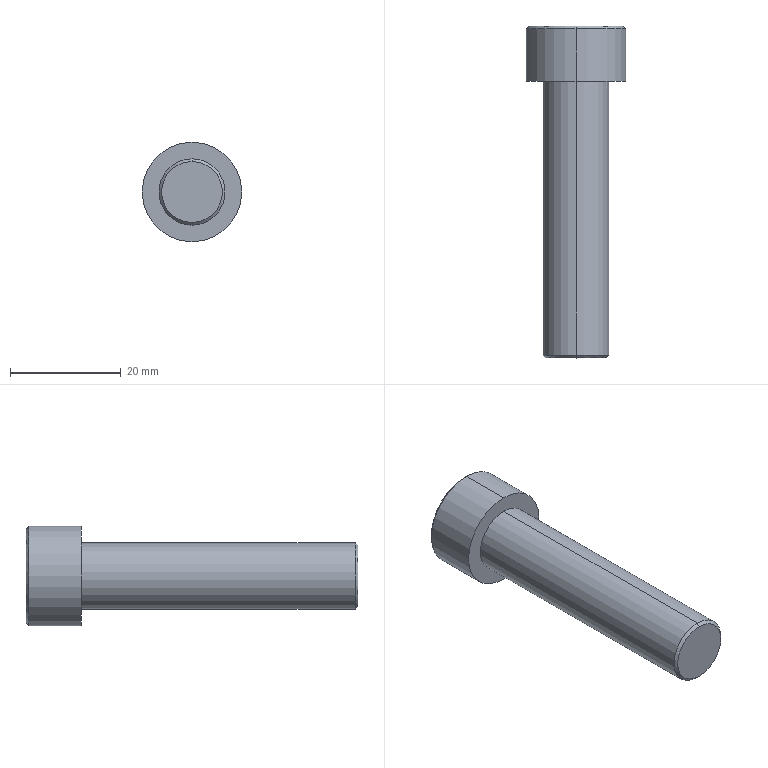Part | SolidWorks | features Chamfer 1, Extrusion 1, ICE 1 | 1 solid | 11 faces | box 18 x 60 x 18 mm | volume 8188 mm3 | cone 4 | cylinder 4 | plane 3 | commonest cylinder face diameters 12 x2 18 x2
STEP:
#1=CARTESIAN_POINT('',(0.,35.,8.5));
#2=VERTEX_POINT('',#1);
#3=CARTESIAN_POINT('',(0.,35.,-8.5));
#4=VERTEX_POINT('',#3);
#5=CARTESIAN_POINT('',(0.,35.,0.));
#6=DIRECTION('',(0.,1.,0.));
#7=DIRECTION('',(0.,0.,1.));
#8=AXIS2_PLACEMENT_3D('',#5,#6,#7);
#9=CIRCLE('',#8,8.5);
#10=EDGE_CURVE('',#2,#4,#9,.T.);
#11=ORIENTED_EDGE('',*,*,#10,.F.);
#12=CARTESIAN_POINT('',(0.,34.5,9.));
#13=VERTEX_POINT('',#12);
#14=CARTESIAN_POINT('',(0.,35.,8.5));
#15=DIRECTION('',(0.,-0.7071,0.7071));
#16=VECTOR('',#15,1000.);
#17=LINE('',#14,#16);
#18=EDGE_CURVE('',#2,#13,#17,.T.);
#19=ORIENTED_EDGE('',*,*,#18,.T.);
#20=CARTESIAN_POINT('',(0.,34.5,-9.));
#21=VERTEX_POINT('',#20);
#22=CARTESIAN_POINT('',(0.,34.5,0.));
#23=DIRECTION('',(0.,-1.,0.));
#24=DIRECTION('',(0.,0.,1.));
#25=AXIS2_PLACEMENT_3D('',#22,#23,#24);
#26=CIRCLE('',#25,9.);
#27=EDGE_CURVE('',#21,#13,#26,.T.);
#28=ORIENTED_EDGE('',*,*,#27,.F.);
#29=CARTESIAN_POINT('',(0.,35.,-8.5));
#30=DIRECTION('',(0.,-0.7071,-0.7071));
#31=VECTOR('',#30,1000.);
#32=LINE('',#29,#31);
#33=EDGE_CURVE('',#4,#21,#32,.T.);
#34=ORIENTED_EDGE('',*,*,#33,.F.);
#35=EDGE_LOOP('',(#11,#19,#28,#34));
#36=FACE_OUTER_BOUND('',#35,.T.);
#37=CARTESIAN_POINT('',(0.,35.,0.));
#38=DIRECTION('',(0.,-1.,0.));
#39=DIRECTION('',(0.,0.,-1.));
#40=AXIS2_PLACEMENT_3D('',#37,#38,#39);
#41=CONICAL_SURFACE('',#40,8.5,0.7854);
#42=ADVANCED_FACE('',(#36),#41,.T.);
#43=CARTESIAN_POINT('',(0.,-25.,-5.5));
#44=VERTEX_POINT('',#43);
#45=CARTESIAN_POINT('',(0.,-25.,5.5));
#46=VERTEX_POINT('',#45);
#47=CARTESIAN_POINT('',(0.,-25.,0.));
#48=DIRECTION('',(0.,-1.,0.));
#49=DIRECTION('',(0.,0.,1.));
#50=AXIS2_PLACEMENT_3D('',#47,#48,#49);
#51=CIRCLE('',#50,5.5);
#52=EDGE_CURVE('',#44,#46,#51,.T.);
#53=ORIENTED_EDGE('',*,*,#52,.F.);
#54=CARTESIAN_POINT('',(0.,-24.5,-6.));
#55=VERTEX_POINT('',#54);
#56=CARTESIAN_POINT('',(0.,-24.5,-6.));
#57=DIRECTION('',(0.,0.7071,-0.7071));
#58=VECTOR('',#57,1000.);
#59=LINE('',#56,#58);
#60=EDGE_CURVE('',#44,#55,#59,.T.);
#61=ORIENTED_EDGE('',*,*,#60,.T.);
#62=CARTESIAN_POINT('',(0.,-24.5,6.));
#63=VERTEX_POINT('',#62);
#64=CARTESIAN_POINT('',(0.,-24.5,0.));
#65=DIRECTION('',(0.,1.,0.));
#66=DIRECTION('',(0.,0.,1.));
#67=AXIS2_PLACEMENT_3D('',#64,#65,#66);
#68=CIRCLE('',#67,6.);
#69=EDGE_CURVE('',#63,#55,#68,.T.);
#70=ORIENTED_EDGE('',*,*,#69,.F.);
#71=CARTESIAN_POINT('',(0.,-24.5,6.));
#72=DIRECTION('',(0.,0.7071,0.7071));
#73=VECTOR('',#72,1000.);
#74=LINE('',#71,#73);
#75=EDGE_CURVE('',#46,#63,#74,.T.);
#76=ORIENTED_EDGE('',*,*,#75,.F.);
#77=EDGE_LOOP('',(#53,#61,#70,#76));
#78=FACE_OUTER_BOUND('',#77,.T.);
#79=CARTESIAN_POINT('',(0.,-24.5,0.));
#80=DIRECTION('',(0.,1.,0.));
#81=DIRECTION('',(0.,0.,1.));
#82=AXIS2_PLACEMENT_3D('',#79,#80,#81);
#83=CONICAL_SURFACE('',#82,6.,0.7854);
#84=ADVANCED_FACE('',(#78),#83,.T.);
#85=ORIENTED_EDGE('',*,*,#27,.T.);
#86=CARTESIAN_POINT('',(0.,25.,9.));
#87=VERTEX_POINT('',#86);
#88=CARTESIAN_POINT('',(0.,35.,9.));
#89=DIRECTION('',(0.,-1.,0.));
#90=VECTOR('',#89,1000.);
#91=LINE('',#88,#90);
#92=EDGE_CURVE('',#13,#87,#91,.T.);
#93=ORIENTED_EDGE('',*,*,#92,.T.);
#94=CARTESIAN_POINT('',(0.,25.,-9.));
#95=VERTEX_POINT('',#94);
#96=CARTESIAN_POINT('',(0.,25.,0.));
#97=DIRECTION('',(0.,1.,0.));
#98=DIRECTION('',(0.,0.,1.));
#99=AXIS2_PLACEMENT_3D('',#96,#97,#98);
#100=CIRCLE('',#99,9.);
#101=EDGE_CURVE('',#87,#95,#100,.T.);
#102=ORIENTED_EDGE('',*,*,#101,.T.);
#103=CARTESIAN_POINT('',(0.,35.,-9.));
#104=DIRECTION('',(0.,-1.,0.));
#105=VECTOR('',#104,1000.);
#106=LINE('',#103,#105);
#107=EDGE_CURVE('',#21,#95,#106,.T.);
#108=ORIENTED_EDGE('',*,*,#107,.F.);
#109=EDGE_LOOP('',(#85,#93,#102,#108));
#110=FACE_OUTER_BOUND('',#109,.T.);
#111=CARTESIAN_POINT('',(0.,35.,0.));
#112=DIRECTION('',(0.,-1.,0.));
#113=DIRECTION('',(0.,0.,-1.));
#114=AXIS2_PLACEMENT_3D('',#111,#112,#113);
#115=CYLINDRICAL_SURFACE('',#114,9.);
#116=ADVANCED_FACE('',(#110),#115,.T.);
#117=CARTESIAN_POINT('',(0.,25.,6.));
#118=VERTEX_POINT('',#117);
#119=CARTESIAN_POINT('',(0.,25.,-6.));
#120=VERTEX_POINT('',#119);
#121=CARTESIAN_POINT('',(0.,25.,0.));
#122=DIRECTION('',(0.,1.,0.));
#123=DIRECTION('',(0.,0.,1.));
#124=AXIS2_PLACEMENT_3D('',#121,#122,#123);
#125=CIRCLE('',#124,6.);
#126=EDGE_CURVE('',#118,#120,#125,.T.);
#127=ORIENTED_EDGE('',*,*,#126,.F.);
#128=CARTESIAN_POINT('',(0.,25.,6.));
#129=DIRECTION('',(0.,-1.,0.));
#130=VECTOR('',#129,1000.);
#131=LINE('',#128,#130);
#132=EDGE_CURVE('',#118,#63,#131,.T.);
#133=ORIENTED_EDGE('',*,*,#132,.T.);
#134=ORIENTED_EDGE('',*,*,#69,.T.);
#135=CARTESIAN_POINT('',(0.,25.,-6.));
#136=DIRECTION('',(0.,-1.,0.));
#137=VECTOR('',#136,1000.);
#138=LINE('',#135,#137);
#139=EDGE_CURVE('',#120,#55,#138,.T.);
#140=ORIENTED_EDGE('',*,*,#139,.F.);
#141=EDGE_LOOP('',(#127,#133,#134,#140));
#142=FACE_OUTER_BOUND('',#141,.T.);
#143=CARTESIAN_POINT('',(0.,25.,0.));
#144=DIRECTION('',(0.,-1.,0.));
#145=DIRECTION('',(0.,0.,-1.));
#146=AXIS2_PLACEMENT_3D('',#143,#144,#145);
#147=CYLINDRICAL_SURFACE('',#146,6.);
#148=ADVANCED_FACE('',(#142),#147,.T.);
#149=ORIENTED_EDGE('',*,*,#132,.F.);
#150=CARTESIAN_POINT('',(0.,25.,0.));
#151=DIRECTION('',(0.,1.,0.));
#152=DIRECTION('',(0.,0.,1.));
#153=AXIS2_PLACEMENT_3D('',#150,#151,#152);
#154=CIRCLE('',#153,6.);
#155=EDGE_CURVE('',#120,#118,#154,.T.);
#156=ORIENTED_EDGE('',*,*,#155,.F.);
#157=ORIENTED_EDGE('',*,*,#139,.T.);
#158=CARTESIAN_POINT('',(0.,-24.5,0.));
#159=DIRECTION('',(0.,1.,0.));
#160=DIRECTION('',(0.,0.,1.));
#161=AXIS2_PLACEMENT_3D('',#158,#159,#160);
#162=CIRCLE('',#161,6.);
#163=EDGE_CURVE('',#55,#63,#162,.T.);
#164=ORIENTED_EDGE('',*,*,#163,.T.);
#165=EDGE_LOOP('',(#149,#156,#157,#164));
#166=FACE_OUTER_BOUND('',#165,.T.);
#167=CARTESIAN_POINT('',(0.,25.,0.));
#168=DIRECTION('',(0.,-1.,0.));
#169=DIRECTION('',(0.,0.,-1.));
#170=AXIS2_PLACEMENT_3D('',#167,#168,#169);
#171=CYLINDRICAL_SURFACE('',#170,6.);
#172=ADVANCED_FACE('',(#166),#171,.T.);
#173=CARTESIAN_POINT('',(0.,-25.,0.));
#174=DIRECTION('',(0.,-1.,0.));
#175=DIRECTION('',(0.,0.,1.));
#176=AXIS2_PLACEMENT_3D('',#173,#174,#175);
#177=CIRCLE('',#176,5.5);
#178=EDGE_CURVE('',#46,#44,#177,.T.);
#179=ORIENTED_EDGE('',*,*,#178,.T.);
#180=ORIENTED_EDGE('',*,*,#52,.T.);
#181=EDGE_LOOP('',(#179,#180));
#182=FACE_OUTER_BOUND('',#181,.T.);
#183=CARTESIAN_POINT('',(0.,-25.,0.));
#184=DIRECTION('',(0.,1.,0.));
#185=DIRECTION('',(0.,0.,1.));
#186=AXIS2_PLACEMENT_3D('',#183,#184,#185);
#187=PLANE('',#186);
#188=ADVANCED_FACE('',(#182),#187,.F.);
#189=ORIENTED_EDGE('',*,*,#92,.F.);
#190=CARTESIAN_POINT('',(0.,34.5,0.));
#191=DIRECTION('',(0.,-1.,0.));
#192=DIRECTION('',(0.,0.,1.));
#193=AXIS2_PLACEMENT_3D('',#190,#191,#192);
#194=CIRCLE('',#193,9.);
#195=EDGE_CURVE('',#13,#21,#194,.T.);
#196=ORIENTED_EDGE('',*,*,#195,.T.);
#197=ORIENTED_EDGE('',*,*,#107,.T.);
#198=CARTESIAN_POINT('',(0.,25.,0.));
#199=DIRECTION('',(0.,1.,0.));
#200=DIRECTION('',(0.,0.,1.));
#201=AXIS2_PLACEMENT_3D('',#198,#199,#200);
#202=CIRCLE('',#201,9.);
#203=EDGE_CURVE('',#95,#87,#202,.T.);
#204=ORIENTED_EDGE('',*,*,#203,.T.);
#205=EDGE_LOOP('',(#189,#196,#197,#204));
#206=FACE_OUTER_BOUND('',#205,.T.);
#207=CARTESIAN_POINT('',(0.,35.,0.));
#208=DIRECTION('',(0.,-1.,0.));
#209=DIRECTION('',(0.,0.,-1.));
#210=AXIS2_PLACEMENT_3D('',#207,#208,#209);
#211=CYLINDRICAL_SURFACE('',#210,9.);
#212=ADVANCED_FACE('',(#206),#211,.T.);
#213=CARTESIAN_POINT('',(0.,35.,0.));
#214=DIRECTION('',(0.,1.,0.));
#215=DIRECTION('',(0.,0.,1.));
#216=AXIS2_PLACEMENT_3D('',#213,#214,#215);
#217=CIRCLE('',#216,8.5);
#218=EDGE_CURVE('',#4,#2,#217,.T.);
#219=ORIENTED_EDGE('',*,*,#218,.T.);
#220=ORIENTED_EDGE('',*,*,#10,.T.);
#221=EDGE_LOOP('',(#219,#220));
#222=FACE_OUTER_BOUND('',#221,.T.);
#223=CARTESIAN_POINT('',(0.,35.,0.));
#224=DIRECTION('',(0.,1.,0.));
#225=DIRECTION('',(0.,0.,1.));
#226=AXIS2_PLACEMENT_3D('',#223,#224,#225);
#227=PLANE('',#226);
#228=ADVANCED_FACE('',(#222),#227,.T.);
#229=ORIENTED_EDGE('',*,*,#155,.T.);
#230=ORIENTED_EDGE('',*,*,#126,.T.);
#231=EDGE_LOOP('',(#229,#230));
#232=FACE_BOUND('',#231,.T.);
#233=ORIENTED_EDGE('',*,*,#203,.F.);
#234=ORIENTED_EDGE('',*,*,#101,.F.);
#235=EDGE_LOOP('',(#233,#234));
#236=FACE_OUTER_BOUND('',#235,.T.);
#237=CARTESIAN_POINT('',(0.,25.,0.));
#238=DIRECTION('',(0.,1.,0.));
#239=DIRECTION('',(0.,0.,1.));
#240=AXIS2_PLACEMENT_3D('',#237,#238,#239);
#241=PLANE('',#240);
#242=ADVANCED_FACE('',(#232,#236),#241,.F.);
#243=ORIENTED_EDGE('',*,*,#60,.F.);
#244=ORIENTED_EDGE('',*,*,#178,.F.);
#245=ORIENTED_EDGE('',*,*,#75,.T.);
#246=ORIENTED_EDGE('',*,*,#163,.F.);
#247=EDGE_LOOP('',(#243,#244,#245,#246));
#248=FACE_OUTER_BOUND('',#247,.T.);
#249=CARTESIAN_POINT('',(0.,-24.5,0.));
#250=DIRECTION('',(0.,1.,0.));
#251=DIRECTION('',(0.,0.,1.));
#252=AXIS2_PLACEMENT_3D('',#249,#250,#251);
#253=CONICAL_SURFACE('',#252,6.,0.7854);
#254=ADVANCED_FACE('',(#248),#253,.T.);
#255=ORIENTED_EDGE('',*,*,#18,.F.);
#256=ORIENTED_EDGE('',*,*,#218,.F.);
#257=ORIENTED_EDGE('',*,*,#33,.T.);
#258=ORIENTED_EDGE('',*,*,#195,.F.);
#259=EDGE_LOOP('',(#255,#256,#257,#258));
#260=FACE_OUTER_BOUND('',#259,.T.);
#261=CARTESIAN_POINT('',(0.,35.,0.));
#262=DIRECTION('',(0.,-1.,0.));
#263=DIRECTION('',(0.,0.,-1.));
#264=AXIS2_PLACEMENT_3D('',#261,#262,#263);
#265=CONICAL_SURFACE('',#264,8.5,0.7854);
#266=ADVANCED_FACE('',(#260),#265,.T.);
#267=CLOSED_SHELL('',(#42,#84,#116,#148,#172,#188,#212,#228,#242,#254,#266));
#268=MANIFOLD_SOLID_BREP('',#267);
#269=CARTESIAN_POINT('',(0.,0.,0.));
#270=DIRECTION('',(0.,0.,1.));
#271=DIRECTION('',(1.,0.,0.));
#272=AXIS2_PLACEMENT_3D('',#269,#270,#271);
#273=(LENGTH_UNIT()NAMED_UNIT(*)SI_UNIT(.MILLI.,.METRE.));
#274=UNCERTAINTY_MEASURE_WITH_UNIT(LENGTH_MEASURE(0.00001),#273,'','');
#275=(NAMED_UNIT(*)PLANE_ANGLE_UNIT()SI_UNIT($,.RADIAN.));
#276=(NAMED_UNIT(*)SI_UNIT($,.STERADIAN.)SOLID_ANGLE_UNIT());
#277=(GEOMETRIC_REPRESENTATION_CONTEXT(3)GLOBAL_UNCERTAINTY_ASSIGNED_CONTEXT((#274))GLOBAL_UNIT_ASSIGNED_CONTEXT((#273,#275,#276))REPRESENTATION_CONTEXT('',''));
#278=ADVANCED_BREP_SHAPE_REPRESENTATION('',(#268,#272),#277);